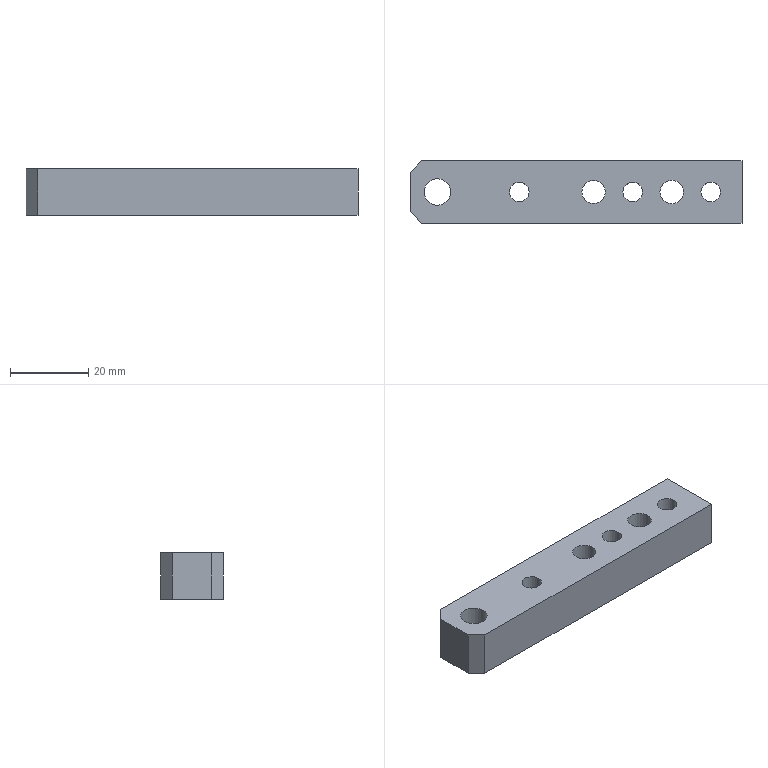Part | NX | features BREP 1 | 1 solid | 14 faces | box 85 x 16 x 12 mm | volume 14391 mm3 | plane 8 | cylinder 6 | commonest cylinder face diameters 5 x3 6 x2 6.8 x1
STEP:
#1=CARTESIAN_POINT('',(42.5,8.,12.));
#2=VERTEX_POINT('',#1);
#3=CARTESIAN_POINT('',(-39.5,8.,12.));
#4=VERTEX_POINT('',#3);
#5=CARTESIAN_POINT('',(0.,8.,12.));
#6=DIRECTION('',(-1.,0.,0.));
#7=VECTOR('',#6,1000.);
#8=LINE('',#5,#7);
#9=EDGE_CURVE('',#2,#4,#8,.T.);
#10=ORIENTED_EDGE('',*,*,#9,.T.);
#11=CARTESIAN_POINT('',(-42.5,5.,12.));
#12=VERTEX_POINT('',#11);
#13=CARTESIAN_POINT('',(-39.5,8.,12.));
#14=DIRECTION('',(-0.7071,-0.7071,0.));
#15=VECTOR('',#14,1000.);
#16=LINE('',#13,#15);
#17=EDGE_CURVE('',#4,#12,#16,.T.);
#18=ORIENTED_EDGE('',*,*,#17,.T.);
#19=CARTESIAN_POINT('',(-42.5,-5.,12.));
#20=VERTEX_POINT('',#19);
#21=CARTESIAN_POINT('',(-42.5,0.,12.));
#22=DIRECTION('',(0.,-1.,0.));
#23=VECTOR('',#22,1000.);
#24=LINE('',#21,#23);
#25=EDGE_CURVE('',#12,#20,#24,.T.);
#26=ORIENTED_EDGE('',*,*,#25,.T.);
#27=CARTESIAN_POINT('',(-39.5,-8.,12.));
#28=VERTEX_POINT('',#27);
#29=CARTESIAN_POINT('',(-42.5,-5.,12.));
#30=DIRECTION('',(0.7071,-0.7071,0.));
#31=VECTOR('',#30,1000.);
#32=LINE('',#29,#31);
#33=EDGE_CURVE('',#20,#28,#32,.T.);
#34=ORIENTED_EDGE('',*,*,#33,.T.);
#35=CARTESIAN_POINT('',(42.5,-8.,12.));
#36=VERTEX_POINT('',#35);
#37=CARTESIAN_POINT('',(0.,-8.,12.));
#38=DIRECTION('',(1.,0.,0.));
#39=VECTOR('',#38,1000.);
#40=LINE('',#37,#39);
#41=EDGE_CURVE('',#28,#36,#40,.T.);
#42=ORIENTED_EDGE('',*,*,#41,.T.);
#43=CARTESIAN_POINT('',(42.5,0.,12.));
#44=DIRECTION('',(0.,1.,0.));
#45=VECTOR('',#44,1000.);
#46=LINE('',#43,#45);
#47=EDGE_CURVE('',#36,#2,#46,.T.);
#48=ORIENTED_EDGE('',*,*,#47,.T.);
#49=EDGE_LOOP('',(#10,#18,#26,#34,#42,#48));
#50=FACE_BOUND('',#49,.T.);
#51=CARTESIAN_POINT('',(27.5,0.,12.));
#52=VERTEX_POINT('',#51);
#53=CARTESIAN_POINT('',(24.5,0.,12.));
#54=DIRECTION('',(0.,0.,-1.));
#55=DIRECTION('',(1.,0.,0.));
#56=AXIS2_PLACEMENT_3D('',#53,#54,#55);
#57=CIRCLE('',#56,3.);
#58=EDGE_CURVE('',#52,#52,#57,.T.);
#59=ORIENTED_EDGE('',*,*,#58,.T.);
#60=EDGE_LOOP('',(#59));
#61=FACE_BOUND('',#60,.T.);
#62=CARTESIAN_POINT('',(7.5,0.,12.));
#63=VERTEX_POINT('',#62);
#64=CARTESIAN_POINT('',(4.5,0.,12.));
#65=DIRECTION('',(0.,0.,-1.));
#66=DIRECTION('',(1.,0.,0.));
#67=AXIS2_PLACEMENT_3D('',#64,#65,#66);
#68=CIRCLE('',#67,3.);
#69=EDGE_CURVE('',#63,#63,#68,.T.);
#70=ORIENTED_EDGE('',*,*,#69,.T.);
#71=EDGE_LOOP('',(#70));
#72=FACE_BOUND('',#71,.T.);
#73=CARTESIAN_POINT('',(17.,0.,12.));
#74=VERTEX_POINT('',#73);
#75=CARTESIAN_POINT('',(14.5,0.,12.));
#76=DIRECTION('',(0.,0.,-1.));
#77=DIRECTION('',(1.,0.,0.));
#78=AXIS2_PLACEMENT_3D('',#75,#76,#77);
#79=CIRCLE('',#78,2.5);
#80=EDGE_CURVE('',#74,#74,#79,.T.);
#81=ORIENTED_EDGE('',*,*,#80,.T.);
#82=EDGE_LOOP('',(#81));
#83=FACE_BOUND('',#82,.T.);
#84=CARTESIAN_POINT('',(37.,0.,12.));
#85=VERTEX_POINT('',#84);
#86=CARTESIAN_POINT('',(34.5,0.,12.));
#87=DIRECTION('',(0.,0.,-1.));
#88=DIRECTION('',(1.,0.,0.));
#89=AXIS2_PLACEMENT_3D('',#86,#87,#88);
#90=CIRCLE('',#89,2.5);
#91=EDGE_CURVE('',#85,#85,#90,.T.);
#92=ORIENTED_EDGE('',*,*,#91,.T.);
#93=EDGE_LOOP('',(#92));
#94=FACE_BOUND('',#93,.T.);
#95=CARTESIAN_POINT('',(-38.9,0.,12.));
#96=VERTEX_POINT('',#95);
#97=CARTESIAN_POINT('',(-35.5,0.,12.));
#98=DIRECTION('',(0.,0.,-1.));
#99=DIRECTION('',(-1.,0.,0.));
#100=AXIS2_PLACEMENT_3D('',#97,#98,#99);
#101=CIRCLE('',#100,3.4);
#102=EDGE_CURVE('',#96,#96,#101,.T.);
#103=ORIENTED_EDGE('',*,*,#102,.T.);
#104=EDGE_LOOP('',(#103));
#105=FACE_BOUND('',#104,.T.);
#106=CARTESIAN_POINT('',(-12.,0.,12.));
#107=VERTEX_POINT('',#106);
#108=CARTESIAN_POINT('',(-14.5,0.,12.));
#109=DIRECTION('',(0.,0.,-1.));
#110=DIRECTION('',(1.,0.,0.));
#111=AXIS2_PLACEMENT_3D('',#108,#109,#110);
#112=CIRCLE('',#111,2.5);
#113=EDGE_CURVE('',#107,#107,#112,.T.);
#114=ORIENTED_EDGE('',*,*,#113,.T.);
#115=EDGE_LOOP('',(#114));
#116=FACE_BOUND('',#115,.T.);
#117=CARTESIAN_POINT('',(0.,0.,12.));
#118=DIRECTION('',(0.,0.,1.));
#119=DIRECTION('',(-1.,0.,0.));
#120=AXIS2_PLACEMENT_3D('',#117,#118,#119);
#121=PLANE('',#120);
#122=ADVANCED_FACE('',(#50,#61,#72,#83,#94,#105,#116),#121,.T.);
#123=CARTESIAN_POINT('',(-39.5,8.,0.));
#124=VERTEX_POINT('',#123);
#125=CARTESIAN_POINT('',(-39.5,8.,12.));
#126=DIRECTION('',(0.,0.,1.));
#127=VECTOR('',#126,1000.);
#128=LINE('',#125,#127);
#129=EDGE_CURVE('',#124,#4,#128,.T.);
#130=ORIENTED_EDGE('',*,*,#129,.F.);
#131=CARTESIAN_POINT('',(-42.5,5.,0.));
#132=VERTEX_POINT('',#131);
#133=CARTESIAN_POINT('',(-42.5,5.,0.));
#134=DIRECTION('',(0.7071,0.7071,0.));
#135=VECTOR('',#134,1000.);
#136=LINE('',#133,#135);
#137=EDGE_CURVE('',#132,#124,#136,.T.);
#138=ORIENTED_EDGE('',*,*,#137,.F.);
#139=CARTESIAN_POINT('',(-42.5,5.,12.));
#140=DIRECTION('',(0.,0.,-1.));
#141=VECTOR('',#140,1000.);
#142=LINE('',#139,#141);
#143=EDGE_CURVE('',#12,#132,#142,.T.);
#144=ORIENTED_EDGE('',*,*,#143,.F.);
#145=ORIENTED_EDGE('',*,*,#17,.F.);
#146=EDGE_LOOP('',(#130,#138,#144,#145));
#147=FACE_BOUND('',#146,.T.);
#148=CARTESIAN_POINT('',(-42.5,5.,12.));
#149=DIRECTION('',(0.7071,-0.7071,0.));
#150=DIRECTION('',(-0.7071,-0.7071,0.));
#151=AXIS2_PLACEMENT_3D('',#148,#149,#150);
#152=PLANE('',#151);
#153=ADVANCED_FACE('',(#147),#152,.F.);
#154=ORIENTED_EDGE('',*,*,#129,.T.);
#155=ORIENTED_EDGE('',*,*,#9,.F.);
#156=CARTESIAN_POINT('',(42.5,8.,0.));
#157=VERTEX_POINT('',#156);
#158=CARTESIAN_POINT('',(42.5,8.,12.));
#159=DIRECTION('',(0.,0.,1.));
#160=VECTOR('',#159,1000.);
#161=LINE('',#158,#160);
#162=EDGE_CURVE('',#157,#2,#161,.T.);
#163=ORIENTED_EDGE('',*,*,#162,.F.);
#164=CARTESIAN_POINT('',(-42.5,8.,0.));
#165=DIRECTION('',(1.,0.,0.));
#166=VECTOR('',#165,1000.);
#167=LINE('',#164,#166);
#168=EDGE_CURVE('',#124,#157,#167,.T.);
#169=ORIENTED_EDGE('',*,*,#168,.F.);
#170=EDGE_LOOP('',(#154,#155,#163,#169));
#171=FACE_BOUND('',#170,.T.);
#172=CARTESIAN_POINT('',(-42.5,8.,12.));
#173=DIRECTION('',(0.,-1.,0.));
#174=DIRECTION('',(0.,0.,1.));
#175=AXIS2_PLACEMENT_3D('',#172,#173,#174);
#176=PLANE('',#175);
#177=ADVANCED_FACE('',(#171),#176,.F.);
#178=ORIENTED_EDGE('',*,*,#162,.T.);
#179=ORIENTED_EDGE('',*,*,#47,.F.);
#180=CARTESIAN_POINT('',(42.5,-8.,0.));
#181=VERTEX_POINT('',#180);
#182=CARTESIAN_POINT('',(42.5,-8.,12.));
#183=DIRECTION('',(0.,0.,1.));
#184=VECTOR('',#183,1000.);
#185=LINE('',#182,#184);
#186=EDGE_CURVE('',#181,#36,#185,.T.);
#187=ORIENTED_EDGE('',*,*,#186,.F.);
#188=CARTESIAN_POINT('',(42.5,8.,0.));
#189=DIRECTION('',(0.,-1.,0.));
#190=VECTOR('',#189,1000.);
#191=LINE('',#188,#190);
#192=EDGE_CURVE('',#157,#181,#191,.T.);
#193=ORIENTED_EDGE('',*,*,#192,.F.);
#194=EDGE_LOOP('',(#178,#179,#187,#193));
#195=FACE_BOUND('',#194,.T.);
#196=CARTESIAN_POINT('',(42.5,8.,12.));
#197=DIRECTION('',(-1.,0.,0.));
#198=DIRECTION('',(0.,0.,-1.));
#199=AXIS2_PLACEMENT_3D('',#196,#197,#198);
#200=PLANE('',#199);
#201=ADVANCED_FACE('',(#195),#200,.F.);
#202=CARTESIAN_POINT('',(-39.5,-8.,0.));
#203=VERTEX_POINT('',#202);
#204=CARTESIAN_POINT('',(-39.5,-8.,12.));
#205=DIRECTION('',(0.,0.,1.));
#206=VECTOR('',#205,1000.);
#207=LINE('',#204,#206);
#208=EDGE_CURVE('',#203,#28,#207,.T.);
#209=ORIENTED_EDGE('',*,*,#208,.F.);
#210=CARTESIAN_POINT('',(-42.5,-8.,0.));
#211=DIRECTION('',(-1.,0.,0.));
#212=VECTOR('',#211,1000.);
#213=LINE('',#210,#212);
#214=EDGE_CURVE('',#181,#203,#213,.T.);
#215=ORIENTED_EDGE('',*,*,#214,.F.);
#216=ORIENTED_EDGE('',*,*,#186,.T.);
#217=ORIENTED_EDGE('',*,*,#41,.F.);
#218=EDGE_LOOP('',(#209,#215,#216,#217));
#219=FACE_BOUND('',#218,.T.);
#220=CARTESIAN_POINT('',(-42.5,-8.,12.));
#221=DIRECTION('',(0.,1.,0.));
#222=DIRECTION('',(0.,0.,-1.));
#223=AXIS2_PLACEMENT_3D('',#220,#221,#222);
#224=PLANE('',#223);
#225=ADVANCED_FACE('',(#219),#224,.F.);
#226=CARTESIAN_POINT('',(-42.5,-5.,0.));
#227=VERTEX_POINT('',#226);
#228=CARTESIAN_POINT('',(-42.5,-5.,12.));
#229=DIRECTION('',(0.,0.,1.));
#230=VECTOR('',#229,1000.);
#231=LINE('',#228,#230);
#232=EDGE_CURVE('',#227,#20,#231,.T.);
#233=ORIENTED_EDGE('',*,*,#232,.F.);
#234=CARTESIAN_POINT('',(-39.5,-8.,0.));
#235=DIRECTION('',(-0.7071,0.7071,0.));
#236=VECTOR('',#235,1000.);
#237=LINE('',#234,#236);
#238=EDGE_CURVE('',#203,#227,#237,.T.);
#239=ORIENTED_EDGE('',*,*,#238,.F.);
#240=ORIENTED_EDGE('',*,*,#208,.T.);
#241=ORIENTED_EDGE('',*,*,#33,.F.);
#242=EDGE_LOOP('',(#233,#239,#240,#241));
#243=FACE_BOUND('',#242,.T.);
#244=CARTESIAN_POINT('',(-39.5,-8.,12.));
#245=DIRECTION('',(0.7071,0.7071,0.));
#246=DIRECTION('',(0.7071,-0.7071,0.));
#247=AXIS2_PLACEMENT_3D('',#244,#245,#246);
#248=PLANE('',#247);
#249=ADVANCED_FACE('',(#243),#248,.F.);
#250=ORIENTED_EDGE('',*,*,#232,.T.);
#251=ORIENTED_EDGE('',*,*,#25,.F.);
#252=ORIENTED_EDGE('',*,*,#143,.T.);
#253=CARTESIAN_POINT('',(-42.5,8.,0.));
#254=DIRECTION('',(0.,1.,0.));
#255=VECTOR('',#254,1000.);
#256=LINE('',#253,#255);
#257=EDGE_CURVE('',#227,#132,#256,.T.);
#258=ORIENTED_EDGE('',*,*,#257,.F.);
#259=EDGE_LOOP('',(#250,#251,#252,#258));
#260=FACE_BOUND('',#259,.T.);
#261=CARTESIAN_POINT('',(-42.5,8.,12.));
#262=DIRECTION('',(1.,0.,0.));
#263=DIRECTION('',(0.,0.,1.));
#264=AXIS2_PLACEMENT_3D('',#261,#262,#263);
#265=PLANE('',#264);
#266=ADVANCED_FACE('',(#260),#265,.F.);
#267=ORIENTED_EDGE('',*,*,#58,.F.);
#268=EDGE_LOOP('',(#267));
#269=FACE_BOUND('',#268,.T.);
#270=CARTESIAN_POINT('',(27.5,0.,0.));
#271=VERTEX_POINT('',#270);
#272=CARTESIAN_POINT('',(24.5,0.,0.));
#273=DIRECTION('',(0.,0.,1.));
#274=DIRECTION('',(1.,0.,0.));
#275=AXIS2_PLACEMENT_3D('',#272,#273,#274);
#276=CIRCLE('',#275,3.);
#277=EDGE_CURVE('',#271,#271,#276,.T.);
#278=ORIENTED_EDGE('',*,*,#277,.F.);
#279=EDGE_LOOP('',(#278));
#280=FACE_BOUND('',#279,.T.);
#281=CARTESIAN_POINT('',(24.5,0.,12.));
#282=DIRECTION('',(0.,0.,1.));
#283=DIRECTION('',(-1.,0.,0.));
#284=AXIS2_PLACEMENT_3D('',#281,#282,#283);
#285=CYLINDRICAL_SURFACE('',#284,3.);
#286=ADVANCED_FACE('',(#269,#280),#285,.F.);
#287=ORIENTED_EDGE('',*,*,#69,.F.);
#288=EDGE_LOOP('',(#287));
#289=FACE_BOUND('',#288,.T.);
#290=CARTESIAN_POINT('',(7.5,0.,0.));
#291=VERTEX_POINT('',#290);
#292=CARTESIAN_POINT('',(4.5,0.,0.));
#293=DIRECTION('',(0.,0.,1.));
#294=DIRECTION('',(1.,0.,0.));
#295=AXIS2_PLACEMENT_3D('',#292,#293,#294);
#296=CIRCLE('',#295,3.);
#297=EDGE_CURVE('',#291,#291,#296,.T.);
#298=ORIENTED_EDGE('',*,*,#297,.F.);
#299=EDGE_LOOP('',(#298));
#300=FACE_BOUND('',#299,.T.);
#301=CARTESIAN_POINT('',(4.5,0.,12.));
#302=DIRECTION('',(0.,0.,1.));
#303=DIRECTION('',(-1.,0.,0.));
#304=AXIS2_PLACEMENT_3D('',#301,#302,#303);
#305=CYLINDRICAL_SURFACE('',#304,3.);
#306=ADVANCED_FACE('',(#289,#300),#305,.F.);
#307=ORIENTED_EDGE('',*,*,#80,.F.);
#308=EDGE_LOOP('',(#307));
#309=FACE_BOUND('',#308,.T.);
#310=CARTESIAN_POINT('',(17.,0.,0.));
#311=VERTEX_POINT('',#310);
#312=CARTESIAN_POINT('',(14.5,0.,0.));
#313=DIRECTION('',(0.,0.,1.));
#314=DIRECTION('',(1.,0.,0.));
#315=AXIS2_PLACEMENT_3D('',#312,#313,#314);
#316=CIRCLE('',#315,2.5);
#317=EDGE_CURVE('',#311,#311,#316,.T.);
#318=ORIENTED_EDGE('',*,*,#317,.F.);
#319=EDGE_LOOP('',(#318));
#320=FACE_BOUND('',#319,.T.);
#321=CARTESIAN_POINT('',(14.5,0.,12.));
#322=DIRECTION('',(0.,0.,1.));
#323=DIRECTION('',(-1.,0.,0.));
#324=AXIS2_PLACEMENT_3D('',#321,#322,#323);
#325=CYLINDRICAL_SURFACE('',#324,2.5);
#326=ADVANCED_FACE('',(#309,#320),#325,.F.);
#327=ORIENTED_EDGE('',*,*,#91,.F.);
#328=EDGE_LOOP('',(#327));
#329=FACE_BOUND('',#328,.T.);
#330=CARTESIAN_POINT('',(37.,0.,0.));
#331=VERTEX_POINT('',#330);
#332=CARTESIAN_POINT('',(34.5,0.,0.));
#333=DIRECTION('',(0.,0.,1.));
#334=DIRECTION('',(1.,0.,0.));
#335=AXIS2_PLACEMENT_3D('',#332,#333,#334);
#336=CIRCLE('',#335,2.5);
#337=EDGE_CURVE('',#331,#331,#336,.T.);
#338=ORIENTED_EDGE('',*,*,#337,.F.);
#339=EDGE_LOOP('',(#338));
#340=FACE_BOUND('',#339,.T.);
#341=CARTESIAN_POINT('',(34.5,0.,12.));
#342=DIRECTION('',(0.,0.,1.));
#343=DIRECTION('',(-1.,0.,0.));
#344=AXIS2_PLACEMENT_3D('',#341,#342,#343);
#345=CYLINDRICAL_SURFACE('',#344,2.5);
#346=ADVANCED_FACE('',(#329,#340),#345,.F.);
#347=CARTESIAN_POINT('',(-38.9,0.,0.));
#348=VERTEX_POINT('',#347);
#349=CARTESIAN_POINT('',(-35.5,0.,0.));
#350=DIRECTION('',(0.,0.,1.));
#351=DIRECTION('',(-1.,0.,0.));
#352=AXIS2_PLACEMENT_3D('',#349,#350,#351);
#353=CIRCLE('',#352,3.4);
#354=EDGE_CURVE('',#348,#348,#353,.T.);
#355=ORIENTED_EDGE('',*,*,#354,.F.);
#356=EDGE_LOOP('',(#355));
#357=FACE_BOUND('',#356,.T.);
#358=ORIENTED_EDGE('',*,*,#102,.F.);
#359=EDGE_LOOP('',(#358));
#360=FACE_BOUND('',#359,.T.);
#361=CARTESIAN_POINT('',(-35.5,0.,0.));
#362=DIRECTION('',(0.,0.,-1.));
#363=DIRECTION('',(1.,0.,0.));
#364=AXIS2_PLACEMENT_3D('',#361,#362,#363);
#365=CYLINDRICAL_SURFACE('',#364,3.4);
#366=ADVANCED_FACE('',(#357,#360),#365,.F.);
#367=ORIENTED_EDGE('',*,*,#113,.F.);
#368=EDGE_LOOP('',(#367));
#369=FACE_BOUND('',#368,.T.);
#370=CARTESIAN_POINT('',(-12.,0.,0.));
#371=VERTEX_POINT('',#370);
#372=CARTESIAN_POINT('',(-14.5,0.,0.));
#373=DIRECTION('',(0.,0.,1.));
#374=DIRECTION('',(1.,0.,0.));
#375=AXIS2_PLACEMENT_3D('',#372,#373,#374);
#376=CIRCLE('',#375,2.5);
#377=EDGE_CURVE('',#371,#371,#376,.T.);
#378=ORIENTED_EDGE('',*,*,#377,.F.);
#379=EDGE_LOOP('',(#378));
#380=FACE_BOUND('',#379,.T.);
#381=CARTESIAN_POINT('',(-14.5,0.,12.));
#382=DIRECTION('',(0.,0.,1.));
#383=DIRECTION('',(-1.,0.,0.));
#384=AXIS2_PLACEMENT_3D('',#381,#382,#383);
#385=CYLINDRICAL_SURFACE('',#384,2.5);
#386=ADVANCED_FACE('',(#369,#380),#385,.F.);
#387=ORIENTED_EDGE('',*,*,#238,.T.);
#388=ORIENTED_EDGE('',*,*,#257,.T.);
#389=ORIENTED_EDGE('',*,*,#137,.T.);
#390=ORIENTED_EDGE('',*,*,#168,.T.);
#391=ORIENTED_EDGE('',*,*,#192,.T.);
#392=ORIENTED_EDGE('',*,*,#214,.T.);
#393=EDGE_LOOP('',(#387,#388,#389,#390,#391,#392));
#394=FACE_BOUND('',#393,.T.);
#395=ORIENTED_EDGE('',*,*,#277,.T.);
#396=EDGE_LOOP('',(#395));
#397=FACE_BOUND('',#396,.T.);
#398=ORIENTED_EDGE('',*,*,#297,.T.);
#399=EDGE_LOOP('',(#398));
#400=FACE_BOUND('',#399,.T.);
#401=ORIENTED_EDGE('',*,*,#317,.T.);
#402=EDGE_LOOP('',(#401));
#403=FACE_BOUND('',#402,.T.);
#404=ORIENTED_EDGE('',*,*,#337,.T.);
#405=EDGE_LOOP('',(#404));
#406=FACE_BOUND('',#405,.T.);
#407=ORIENTED_EDGE('',*,*,#354,.T.);
#408=EDGE_LOOP('',(#407));
#409=FACE_BOUND('',#408,.T.);
#410=ORIENTED_EDGE('',*,*,#377,.T.);
#411=EDGE_LOOP('',(#410));
#412=FACE_BOUND('',#411,.T.);
#413=CARTESIAN_POINT('',(0.,0.,0.));
#414=DIRECTION('',(0.,0.,1.));
#415=DIRECTION('',(-1.,0.,0.));
#416=AXIS2_PLACEMENT_3D('',#413,#414,#415);
#417=PLANE('',#416);
#418=ADVANCED_FACE('',(#394,#397,#400,#403,#406,#409,#412),#417,.F.);
#419=CLOSED_SHELL('',(#122,#153,#177,#201,#225,#249,#266,#286,#306,#326,#346,#366,#386,#418));
#420=MANIFOLD_SOLID_BREP('',#419);
#421=(LENGTH_UNIT()NAMED_UNIT(*)SI_UNIT(.MILLI.,.METRE.));
#422=UNCERTAINTY_MEASURE_WITH_UNIT(LENGTH_MEASURE(0.00001),#421,'','');
#423=(NAMED_UNIT(*)PLANE_ANGLE_UNIT()SI_UNIT($,.RADIAN.));
#424=(NAMED_UNIT(*)SI_UNIT($,.STERADIAN.)SOLID_ANGLE_UNIT());
#425=(GEOMETRIC_REPRESENTATION_CONTEXT(3)GLOBAL_UNCERTAINTY_ASSIGNED_CONTEXT((#422))GLOBAL_UNIT_ASSIGNED_CONTEXT((#421,#423,#424))REPRESENTATION_CONTEXT('',''));
#426=ADVANCED_BREP_SHAPE_REPRESENTATION('',(#420),#425);